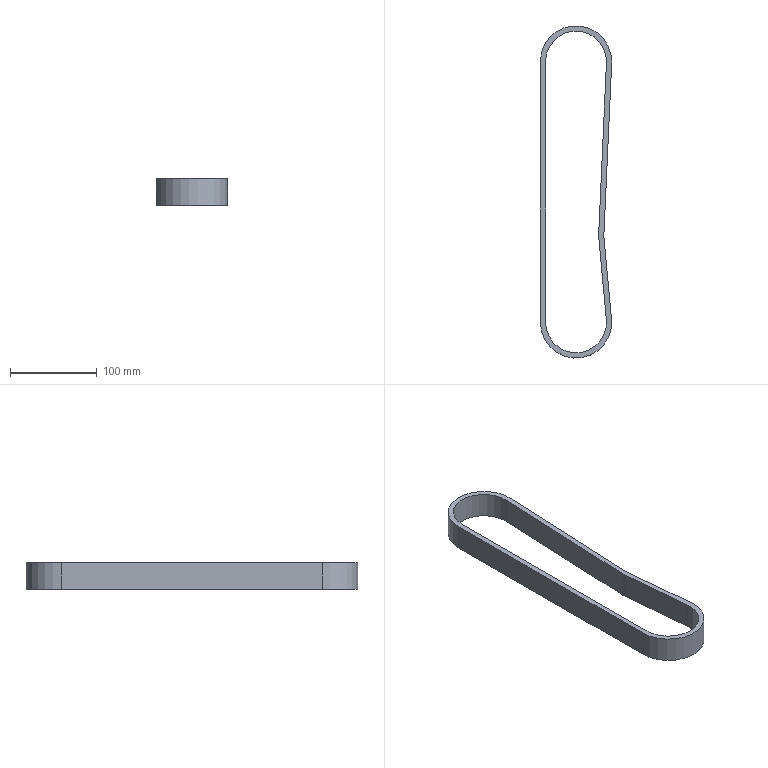Part | STEP file | belt 3-4^longitudinal seal film pull assembly 2 | 1 solid | 16 faces | box 82 x 382 x 30 mm | volume 151088 mm3 | cylinder 8 | plane 8 | commonest cylinder face diameters 40 x2 52 x2 70 x2 82 x2
STEP:
#1=CARTESIAN_POINT('',(0.,0.,0.));
#2=DIRECTION('',(0.,0.,1.));
#3=DIRECTION('',(1.,0.,0.));
#4=AXIS2_PLACEMENT_3D('',#1,#2,#3);
#5=CARTESIAN_POINT('',(32.021,100.905,-15.));
#6=VERTEX_POINT('',#5);
#7=CARTESIAN_POINT('',(32.021,100.905,15.));
#8=VERTEX_POINT('',#7);
#9=CARTESIAN_POINT('',(32.021,100.905,15.));
#10=DIRECTION('',(0.,0.,1.));
#11=VECTOR('',#10,1.);
#12=LINE('',#9,#11);
#13=CARTESIAN_POINT('',(52.,100.,15.));
#14=DIRECTION('',(0.,0.,-1.));
#15=DIRECTION('',(-1.,0.,0.));
#16=AXIS2_PLACEMENT_3D('',#13,#14,#15);
#17=CYLINDRICAL_SURFACE('',#16,20.);
#18=CARTESIAN_POINT('',(0.04528,0.));
#19=DIRECTION('',(0.,-1.));
#20=VECTOR('',#19,1.);
#21=LINE('',#18,#20);
#22=(GEOMETRIC_REPRESENTATION_CONTEXT(2)PARAMETRIC_REPRESENTATION_CONTEXT()REPRESENTATION_CONTEXT('',''));
#23=DEFINITIONAL_REPRESENTATION('',(#21),#22);
#24=PCURVE('',#17,#23);
#25=CARTESIAN_POINT('',(27.392,-1.241,15.));
#26=DIRECTION('',(-0.999,0.04527,0.));
#27=DIRECTION('',(-0.04527,-0.999,0.));
#28=AXIS2_PLACEMENT_3D('',#25,#26,#27);
#29=PLANE('',#28);
#30=CARTESIAN_POINT('',(-102.251,0.));
#31=DIRECTION('',(0.,1.));
#32=VECTOR('',#31,1.);
#33=LINE('',#30,#32);
#34=(GEOMETRIC_REPRESENTATION_CONTEXT(2)PARAMETRIC_REPRESENTATION_CONTEXT()REPRESENTATION_CONTEXT('',''));
#35=DEFINITIONAL_REPRESENTATION('',(#33),#34);
#36=PCURVE('',#29,#35);
#37=SURFACE_CURVE('',#12,(#24,#36),.PCURVE_S1.);
#38=EDGE_CURVE('',#6,#8,#37,.T.);
#39=ORIENTED_EDGE('',*,*,#38,.F.);
#40=CARTESIAN_POINT('',(32.,100.,-15.));
#41=VERTEX_POINT('',#40);
#42=CARTESIAN_POINT('',(52.,100.,-15.));
#43=DIRECTION('',(0.,0.,1.));
#44=DIRECTION('',(-1.,0.,0.));
#45=AXIS2_PLACEMENT_3D('',#42,#43,#44);
#46=CIRCLE('',#45,20.);
#47=CARTESIAN_POINT('',(6.283,30.));
#48=DIRECTION('',(-1.,0.));
#49=VECTOR('',#48,1.);
#50=LINE('',#47,#49);
#51=(GEOMETRIC_REPRESENTATION_CONTEXT(2)PARAMETRIC_REPRESENTATION_CONTEXT()REPRESENTATION_CONTEXT('',''));
#52=DEFINITIONAL_REPRESENTATION('',(#50),#51);
#53=PCURVE('',#17,#52);
#54=CARTESIAN_POINT('',(0.,0.,-15.));
#55=DIRECTION('',(0.,0.,-1.));
#56=DIRECTION('',(-1.,0.,0.));
#57=AXIS2_PLACEMENT_3D('',#54,#55,#56);
#58=PLANE('',#57);
#59=CARTESIAN_POINT('',(-32.,100.));
#60=CARTESIAN_POINT('',(-32.,65.359));
#61=CARTESIAN_POINT('',(-62.,82.679));
#62=CARTESIAN_POINT('',(-92.,100.));
#63=CARTESIAN_POINT('',(-62.,117.321));
#64=CARTESIAN_POINT('',(-32.,134.641));
#65=CARTESIAN_POINT('',(-32.,100.));
#66=(BOUNDED_CURVE()B_SPLINE_CURVE(2,(#59,#60,#61,#62,#63,#64,#65),.UNSPECIFIED.,.T.,.F.)B_SPLINE_CURVE_WITH_KNOTS((1,2,2,2,2,1),(-2.094,0.,2.094,4.189,6.283,8.378),.UNSPECIFIED.)CURVE()GEOMETRIC_REPRESENTATION_ITEM()RATIONAL_B_SPLINE_CURVE((1.,0.5,1.,0.5,1.,0.5,1.))REPRESENTATION_ITEM(''));
#67=(GEOMETRIC_REPRESENTATION_CONTEXT(2)PARAMETRIC_REPRESENTATION_CONTEXT()REPRESENTATION_CONTEXT('',''));
#68=DEFINITIONAL_REPRESENTATION('',(#66),#67);
#69=PCURVE('',#58,#68);
#70=SURFACE_CURVE('',#46,(#53,#69),.PCURVE_S1.);
#71=EDGE_CURVE('',#6,#41,#70,.T.);
#72=ORIENTED_EDGE('',*,*,#71,.T.);
#73=CARTESIAN_POINT('',(32.,100.,15.));
#74=VERTEX_POINT('',#73);
#75=CARTESIAN_POINT('',(32.,100.,15.));
#76=DIRECTION('',(0.,0.,-1.));
#77=VECTOR('',#76,1.);
#78=LINE('',#75,#77);
#79=CARTESIAN_POINT('',(0.,0.));
#80=DIRECTION('',(0.,1.));
#81=VECTOR('',#80,1.);
#82=LINE('',#79,#81);
#83=(GEOMETRIC_REPRESENTATION_CONTEXT(2)PARAMETRIC_REPRESENTATION_CONTEXT()REPRESENTATION_CONTEXT('',''));
#84=DEFINITIONAL_REPRESENTATION('',(#82),#83);
#85=PCURVE('',#17,#84);
#86=CARTESIAN_POINT('',(52.,100.,15.));
#87=DIRECTION('',(0.,0.,-1.));
#88=DIRECTION('',(-1.,0.,0.));
#89=AXIS2_PLACEMENT_3D('',#86,#87,#88);
#90=CYLINDRICAL_SURFACE('',#89,20.);
#91=CARTESIAN_POINT('',(6.283,0.));
#92=DIRECTION('',(0.,1.));
#93=VECTOR('',#92,1.);
#94=LINE('',#91,#93);
#95=(GEOMETRIC_REPRESENTATION_CONTEXT(2)PARAMETRIC_REPRESENTATION_CONTEXT()REPRESENTATION_CONTEXT('',''));
#96=DEFINITIONAL_REPRESENTATION('',(#94),#95);
#97=PCURVE('',#90,#96);
#98=SURFACE_CURVE('',#78,(#85,#97),.PCURVE_S1.);
#99=EDGE_CURVE('',#74,#41,#98,.T.);
#100=ORIENTED_EDGE('',*,*,#99,.F.);
#101=CARTESIAN_POINT('',(52.,100.,15.));
#102=DIRECTION('',(0.,0.,1.));
#103=DIRECTION('',(-1.,0.,0.));
#104=AXIS2_PLACEMENT_3D('',#101,#102,#103);
#105=CIRCLE('',#104,20.);
#106=CARTESIAN_POINT('',(6.283,0.));
#107=DIRECTION('',(-1.,0.));
#108=VECTOR('',#107,1.);
#109=LINE('',#106,#108);
#110=(GEOMETRIC_REPRESENTATION_CONTEXT(2)PARAMETRIC_REPRESENTATION_CONTEXT()REPRESENTATION_CONTEXT('',''));
#111=DEFINITIONAL_REPRESENTATION('',(#109),#110);
#112=PCURVE('',#17,#111);
#113=CARTESIAN_POINT('',(0.,0.,15.));
#114=DIRECTION('',(0.,0.,-1.));
#115=DIRECTION('',(-1.,0.,0.));
#116=AXIS2_PLACEMENT_3D('',#113,#114,#115);
#117=PLANE('',#116);
#118=CARTESIAN_POINT('',(-32.,100.));
#119=CARTESIAN_POINT('',(-32.,65.359));
#120=CARTESIAN_POINT('',(-62.,82.679));
#121=CARTESIAN_POINT('',(-92.,100.));
#122=CARTESIAN_POINT('',(-62.,117.321));
#123=CARTESIAN_POINT('',(-32.,134.641));
#124=CARTESIAN_POINT('',(-32.,100.));
#125=(BOUNDED_CURVE()B_SPLINE_CURVE(2,(#118,#119,#120,#121,#122,#123,#124),.UNSPECIFIED.,.T.,.F.)B_SPLINE_CURVE_WITH_KNOTS((1,2,2,2,2,1),(-2.094,0.,2.094,4.189,6.283,8.378),.UNSPECIFIED.)CURVE()GEOMETRIC_REPRESENTATION_ITEM()RATIONAL_B_SPLINE_CURVE((1.,0.5,1.,0.5,1.,0.5,1.))REPRESENTATION_ITEM(''));
#126=(GEOMETRIC_REPRESENTATION_CONTEXT(2)PARAMETRIC_REPRESENTATION_CONTEXT()REPRESENTATION_CONTEXT('',''));
#127=DEFINITIONAL_REPRESENTATION('',(#125),#126);
#128=PCURVE('',#117,#127);
#129=SURFACE_CURVE('',#105,(#112,#128),.PCURVE_S1.);
#130=EDGE_CURVE('',#8,#74,#129,.T.);
#131=ORIENTED_EDGE('',*,*,#130,.F.);
#132=EDGE_LOOP('',(#39,#72,#100,#131));
#133=FACE_BOUND('',#132,.F.);
#134=ADVANCED_FACE('',(#133),#17,.F.);
#135=CARTESIAN_POINT('',(26.111,97.602,15.));
#136=VERTEX_POINT('',#135);
#137=CARTESIAN_POINT('',(26.,100.,15.));
#138=VERTEX_POINT('',#137);
#139=CARTESIAN_POINT('',(52.,100.,15.));
#140=DIRECTION('',(0.,0.,-1.));
#141=DIRECTION('',(-1.,0.,0.));
#142=AXIS2_PLACEMENT_3D('',#139,#140,#141);
#143=CIRCLE('',#142,26.);
#144=CARTESIAN_POINT('',(52.,100.,15.));
#145=DIRECTION('',(0.,0.,-1.));
#146=DIRECTION('',(-1.,0.,0.));
#147=AXIS2_PLACEMENT_3D('',#144,#145,#146);
#148=CYLINDRICAL_SURFACE('',#147,26.);
#149=CARTESIAN_POINT('',(0.,0.));
#150=DIRECTION('',(1.,0.));
#151=VECTOR('',#150,1.);
#152=LINE('',#149,#151);
#153=(GEOMETRIC_REPRESENTATION_CONTEXT(2)PARAMETRIC_REPRESENTATION_CONTEXT()REPRESENTATION_CONTEXT('',''));
#154=DEFINITIONAL_REPRESENTATION('',(#152),#153);
#155=PCURVE('',#148,#154);
#156=CARTESIAN_POINT('',(-52.,100.));
#157=DIRECTION('',(1.,0.));
#158=AXIS2_PLACEMENT_2D('',#156,#157);
#159=CIRCLE('',#158,26.);
#160=(GEOMETRIC_REPRESENTATION_CONTEXT(2)PARAMETRIC_REPRESENTATION_CONTEXT()REPRESENTATION_CONTEXT('',''));
#161=DEFINITIONAL_REPRESENTATION('',(#159),#160);
#162=PCURVE('',#117,#161);
#163=SURFACE_CURVE('',#143,(#155,#162),.PCURVE_S1.);
#164=EDGE_CURVE('',#136,#138,#163,.T.);
#165=ORIENTED_EDGE('',*,*,#164,.T.);
#166=CARTESIAN_POINT('',(26.,100.,-15.));
#167=VERTEX_POINT('',#166);
#168=CARTESIAN_POINT('',(26.,100.,15.));
#169=DIRECTION('',(0.,0.,-1.));
#170=VECTOR('',#169,1.);
#171=LINE('',#168,#170);
#172=CARTESIAN_POINT('',(6.283,0.));
#173=DIRECTION('',(0.,1.));
#174=VECTOR('',#173,1.);
#175=LINE('',#172,#174);
#176=(GEOMETRIC_REPRESENTATION_CONTEXT(2)PARAMETRIC_REPRESENTATION_CONTEXT()REPRESENTATION_CONTEXT('',''));
#177=DEFINITIONAL_REPRESENTATION('',(#175),#176);
#178=PCURVE('',#148,#177);
#179=CARTESIAN_POINT('',(52.,100.,15.));
#180=DIRECTION('',(0.,0.,-1.));
#181=DIRECTION('',(-1.,0.,0.));
#182=AXIS2_PLACEMENT_3D('',#179,#180,#181);
#183=CYLINDRICAL_SURFACE('',#182,26.);
#184=CARTESIAN_POINT('',(0.,0.));
#185=DIRECTION('',(0.,1.));
#186=VECTOR('',#185,1.);
#187=LINE('',#184,#186);
#188=(GEOMETRIC_REPRESENTATION_CONTEXT(2)PARAMETRIC_REPRESENTATION_CONTEXT()REPRESENTATION_CONTEXT('',''));
#189=DEFINITIONAL_REPRESENTATION('',(#187),#188);
#190=PCURVE('',#183,#189);
#191=SURFACE_CURVE('',#171,(#178,#190),.PCURVE_S1.);
#192=EDGE_CURVE('',#138,#167,#191,.T.);
#193=ORIENTED_EDGE('',*,*,#192,.T.);
#194=CARTESIAN_POINT('',(26.111,97.602,-15.));
#195=VERTEX_POINT('',#194);
#196=CARTESIAN_POINT('',(52.,100.,-15.));
#197=DIRECTION('',(0.,0.,-1.));
#198=DIRECTION('',(-1.,0.,0.));
#199=AXIS2_PLACEMENT_3D('',#196,#197,#198);
#200=CIRCLE('',#199,26.);
#201=CARTESIAN_POINT('',(0.,30.));
#202=DIRECTION('',(1.,0.));
#203=VECTOR('',#202,1.);
#204=LINE('',#201,#203);
#205=(GEOMETRIC_REPRESENTATION_CONTEXT(2)PARAMETRIC_REPRESENTATION_CONTEXT()REPRESENTATION_CONTEXT('',''));
#206=DEFINITIONAL_REPRESENTATION('',(#204),#205);
#207=PCURVE('',#148,#206);
#208=CARTESIAN_POINT('',(-52.,100.));
#209=DIRECTION('',(1.,0.));
#210=AXIS2_PLACEMENT_2D('',#208,#209);
#211=CIRCLE('',#210,26.);
#212=(GEOMETRIC_REPRESENTATION_CONTEXT(2)PARAMETRIC_REPRESENTATION_CONTEXT()REPRESENTATION_CONTEXT('',''));
#213=DEFINITIONAL_REPRESENTATION('',(#211),#212);
#214=PCURVE('',#58,#213);
#215=SURFACE_CURVE('',#200,(#207,#214),.PCURVE_S1.);
#216=EDGE_CURVE('',#195,#167,#215,.T.);
#217=ORIENTED_EDGE('',*,*,#216,.F.);
#218=CARTESIAN_POINT('',(26.111,97.602,15.));
#219=DIRECTION('',(0.,0.,1.));
#220=VECTOR('',#219,1.);
#221=LINE('',#218,#220);
#222=CARTESIAN_POINT('',(6.191,0.));
#223=DIRECTION('',(0.,-1.));
#224=VECTOR('',#223,1.);
#225=LINE('',#222,#224);
#226=(GEOMETRIC_REPRESENTATION_CONTEXT(2)PARAMETRIC_REPRESENTATION_CONTEXT()REPRESENTATION_CONTEXT('',''));
#227=DEFINITIONAL_REPRESENTATION('',(#225),#226);
#228=PCURVE('',#148,#227);
#229=CARTESIAN_POINT('',(26.111,97.602,15.));
#230=DIRECTION('',(-0.9957,-0.09222,0.));
#231=DIRECTION('',(0.09222,-0.9957,0.));
#232=AXIS2_PLACEMENT_3D('',#229,#230,#231);
#233=PLANE('',#232);
#234=CARTESIAN_POINT('',(0.,0.));
#235=DIRECTION('',(0.,1.));
#236=VECTOR('',#235,1.);
#237=LINE('',#234,#236);
#238=(GEOMETRIC_REPRESENTATION_CONTEXT(2)PARAMETRIC_REPRESENTATION_CONTEXT()REPRESENTATION_CONTEXT('',''));
#239=DEFINITIONAL_REPRESENTATION('',(#237),#238);
#240=PCURVE('',#233,#239);
#241=SURFACE_CURVE('',#221,(#228,#240),.PCURVE_S1.);
#242=EDGE_CURVE('',#195,#136,#241,.T.);
#243=ORIENTED_EDGE('',*,*,#242,.T.);
#244=EDGE_LOOP('',(#165,#193,#217,#243));
#245=FACE_BOUND('',#244,.T.);
#246=ADVANCED_FACE('',(#245),#148,.T.);
#247=CARTESIAN_POINT('',(-41.,300.,15.));
#248=VERTEX_POINT('',#247);
#249=CARTESIAN_POINT('',(-41.,0.,15.));
#250=VERTEX_POINT('',#249);
#251=CARTESIAN_POINT('',(-41.,0.,15.));
#252=DIRECTION('',(0.,-1.,0.));
#253=VECTOR('',#252,1.);
#254=LINE('',#251,#253);
#255=CARTESIAN_POINT('',(-41.,0.,15.));
#256=DIRECTION('',(1.,0.,0.));
#257=DIRECTION('',(0.,1.,0.));
#258=AXIS2_PLACEMENT_3D('',#255,#256,#257);
#259=PLANE('',#258);
#260=CARTESIAN_POINT('',(0.,0.));
#261=DIRECTION('',(-1.,0.));
#262=VECTOR('',#261,1.);
#263=LINE('',#260,#262);
#264=(GEOMETRIC_REPRESENTATION_CONTEXT(2)PARAMETRIC_REPRESENTATION_CONTEXT()REPRESENTATION_CONTEXT('',''));
#265=DEFINITIONAL_REPRESENTATION('',(#263),#264);
#266=PCURVE('',#259,#265);
#267=CARTESIAN_POINT('',(41.,0.));
#268=DIRECTION('',(0.,-1.));
#269=VECTOR('',#268,1.);
#270=LINE('',#267,#269);
#271=(GEOMETRIC_REPRESENTATION_CONTEXT(2)PARAMETRIC_REPRESENTATION_CONTEXT()REPRESENTATION_CONTEXT('',''));
#272=DEFINITIONAL_REPRESENTATION('',(#270),#271);
#273=PCURVE('',#117,#272);
#274=SURFACE_CURVE('',#254,(#266,#273),.PCURVE_S1.);
#275=EDGE_CURVE('',#248,#250,#274,.T.);
#276=ORIENTED_EDGE('',*,*,#275,.F.);
#277=CARTESIAN_POINT('',(-41.,300.,-15.));
#278=VERTEX_POINT('',#277);
#279=CARTESIAN_POINT('',(-41.,300.,15.));
#280=DIRECTION('',(0.,0.,1.));
#281=VECTOR('',#280,1.);
#282=LINE('',#279,#281);
#283=CARTESIAN_POINT('',(300.,0.));
#284=DIRECTION('',(0.,1.));
#285=VECTOR('',#284,1.);
#286=LINE('',#283,#285);
#287=(GEOMETRIC_REPRESENTATION_CONTEXT(2)PARAMETRIC_REPRESENTATION_CONTEXT()REPRESENTATION_CONTEXT('',''));
#288=DEFINITIONAL_REPRESENTATION('',(#286),#287);
#289=PCURVE('',#259,#288);
#290=CARTESIAN_POINT('',(0.,300.,15.));
#291=DIRECTION('',(0.,0.,-1.));
#292=DIRECTION('',(-1.,0.,0.));
#293=AXIS2_PLACEMENT_3D('',#290,#291,#292);
#294=CYLINDRICAL_SURFACE('',#293,41.);
#295=CARTESIAN_POINT('',(0.,0.));
#296=DIRECTION('',(0.,-1.));
#297=VECTOR('',#296,1.);
#298=LINE('',#295,#297);
#299=(GEOMETRIC_REPRESENTATION_CONTEXT(2)PARAMETRIC_REPRESENTATION_CONTEXT()REPRESENTATION_CONTEXT('',''));
#300=DEFINITIONAL_REPRESENTATION('',(#298),#299);
#301=PCURVE('',#294,#300);
#302=SURFACE_CURVE('',#282,(#289,#301),.PCURVE_S1.);
#303=EDGE_CURVE('',#278,#248,#302,.T.);
#304=ORIENTED_EDGE('',*,*,#303,.F.);
#305=CARTESIAN_POINT('',(-41.,0.,-15.));
#306=VERTEX_POINT('',#305);
#307=CARTESIAN_POINT('',(-41.,0.,-15.));
#308=DIRECTION('',(0.,1.,0.));
#309=VECTOR('',#308,1.);
#310=LINE('',#307,#309);
#311=CARTESIAN_POINT('',(0.,-30.));
#312=DIRECTION('',(1.,0.));
#313=VECTOR('',#312,1.);
#314=LINE('',#311,#313);
#315=(GEOMETRIC_REPRESENTATION_CONTEXT(2)PARAMETRIC_REPRESENTATION_CONTEXT()REPRESENTATION_CONTEXT('',''));
#316=DEFINITIONAL_REPRESENTATION('',(#314),#315);
#317=PCURVE('',#259,#316);
#318=CARTESIAN_POINT('',(41.,0.));
#319=DIRECTION('',(0.,1.));
#320=VECTOR('',#319,1.);
#321=LINE('',#318,#320);
#322=(GEOMETRIC_REPRESENTATION_CONTEXT(2)PARAMETRIC_REPRESENTATION_CONTEXT()REPRESENTATION_CONTEXT('',''));
#323=DEFINITIONAL_REPRESENTATION('',(#321),#322);
#324=PCURVE('',#58,#323);
#325=SURFACE_CURVE('',#310,(#317,#324),.PCURVE_S1.);
#326=EDGE_CURVE('',#306,#278,#325,.T.);
#327=ORIENTED_EDGE('',*,*,#326,.F.);
#328=CARTESIAN_POINT('',(-41.,0.,15.));
#329=DIRECTION('',(0.,0.,-1.));
#330=VECTOR('',#329,1.);
#331=LINE('',#328,#330);
#332=CARTESIAN_POINT('',(0.,0.));
#333=DIRECTION('',(0.,-1.));
#334=VECTOR('',#333,1.);
#335=LINE('',#332,#334);
#336=(GEOMETRIC_REPRESENTATION_CONTEXT(2)PARAMETRIC_REPRESENTATION_CONTEXT()REPRESENTATION_CONTEXT('',''));
#337=DEFINITIONAL_REPRESENTATION('',(#335),#336);
#338=PCURVE('',#259,#337);
#339=CARTESIAN_POINT('',(0.,0.,15.));
#340=DIRECTION('',(0.,0.,-1.));
#341=DIRECTION('',(-1.,0.,0.));
#342=AXIS2_PLACEMENT_3D('',#339,#340,#341);
#343=CYLINDRICAL_SURFACE('',#342,41.);
#344=CARTESIAN_POINT('',(6.283,0.));
#345=DIRECTION('',(0.,1.));
#346=VECTOR('',#345,1.);
#347=LINE('',#344,#346);
#348=(GEOMETRIC_REPRESENTATION_CONTEXT(2)PARAMETRIC_REPRESENTATION_CONTEXT()REPRESENTATION_CONTEXT('',''));
#349=DEFINITIONAL_REPRESENTATION('',(#347),#348);
#350=PCURVE('',#343,#349);
#351=SURFACE_CURVE('',#331,(#338,#350),.PCURVE_S1.);
#352=EDGE_CURVE('',#250,#306,#351,.T.);
#353=ORIENTED_EDGE('',*,*,#352,.F.);
#354=EDGE_LOOP('',(#276,#304,#327,#353));
#355=FACE_BOUND('',#354,.T.);
#356=ADVANCED_FACE('',(#355),#259,.F.);
#357=CARTESIAN_POINT('',(40.825,3.781,-15.));
#358=VERTEX_POINT('',#357);
#359=CARTESIAN_POINT('',(0.,0.,-15.));
#360=DIRECTION('',(0.,0.,1.));
#361=DIRECTION('',(-1.,0.,0.));
#362=AXIS2_PLACEMENT_3D('',#359,#360,#361);
#363=CIRCLE('',#362,41.);
#364=CARTESIAN_POINT('',(6.283,30.));
#365=DIRECTION('',(-1.,0.));
#366=VECTOR('',#365,1.);
#367=LINE('',#364,#366);
#368=(GEOMETRIC_REPRESENTATION_CONTEXT(2)PARAMETRIC_REPRESENTATION_CONTEXT()REPRESENTATION_CONTEXT('',''));
#369=DEFINITIONAL_REPRESENTATION('',(#367),#368);
#370=PCURVE('',#343,#369);
#371=CARTESIAN_POINT('',(41.,0.));
#372=CARTESIAN_POINT('',(41.,-71.014));
#373=CARTESIAN_POINT('',(-20.5,-35.507));
#374=CARTESIAN_POINT('',(-82.,0.));
#375=CARTESIAN_POINT('',(-20.5,35.507));
#376=CARTESIAN_POINT('',(41.,71.014));
#377=CARTESIAN_POINT('',(41.,0.));
#378=(BOUNDED_CURVE()B_SPLINE_CURVE(2,(#371,#372,#373,#374,#375,#376,#377),.UNSPECIFIED.,.T.,.F.)B_SPLINE_CURVE_WITH_KNOTS((1,2,2,2,2,1),(-2.094,0.,2.094,4.189,6.283,8.378),.UNSPECIFIED.)CURVE()GEOMETRIC_REPRESENTATION_ITEM()RATIONAL_B_SPLINE_CURVE((1.,0.5,1.,0.5,1.,0.5,1.))REPRESENTATION_ITEM(''));
#379=(GEOMETRIC_REPRESENTATION_CONTEXT(2)PARAMETRIC_REPRESENTATION_CONTEXT()REPRESENTATION_CONTEXT('',''));
#380=DEFINITIONAL_REPRESENTATION('',(#378),#379);
#381=PCURVE('',#58,#380);
#382=SURFACE_CURVE('',#363,(#370,#381),.PCURVE_S1.);
#383=EDGE_CURVE('',#306,#358,#382,.T.);
#384=ORIENTED_EDGE('',*,*,#383,.T.);
#385=CARTESIAN_POINT('',(40.825,3.781,15.));
#386=VERTEX_POINT('',#385);
#387=CARTESIAN_POINT('',(40.825,3.781,15.));
#388=DIRECTION('',(0.,0.,1.));
#389=VECTOR('',#388,1.);
#390=LINE('',#387,#389);
#391=CARTESIAN_POINT('',(3.049,0.));
#392=DIRECTION('',(0.,-1.));
#393=VECTOR('',#392,1.);
#394=LINE('',#391,#393);
#395=(GEOMETRIC_REPRESENTATION_CONTEXT(2)PARAMETRIC_REPRESENTATION_CONTEXT()REPRESENTATION_CONTEXT('',''));
#396=DEFINITIONAL_REPRESENTATION('',(#394),#395);
#397=PCURVE('',#343,#396);
#398=CARTESIAN_POINT('',(40.825,3.781,15.));
#399=DIRECTION('',(-0.9957,-0.09222,0.));
#400=DIRECTION('',(0.09222,-0.9957,0.));
#401=AXIS2_PLACEMENT_3D('',#398,#399,#400);
#402=PLANE('',#401);
#403=CARTESIAN_POINT('',(0.,0.));
#404=DIRECTION('',(0.,1.));
#405=VECTOR('',#404,1.);
#406=LINE('',#403,#405);
#407=(GEOMETRIC_REPRESENTATION_CONTEXT(2)PARAMETRIC_REPRESENTATION_CONTEXT()REPRESENTATION_CONTEXT('',''));
#408=DEFINITIONAL_REPRESENTATION('',(#406),#407);
#409=PCURVE('',#402,#408);
#410=SURFACE_CURVE('',#390,(#397,#409),.PCURVE_S1.);
#411=EDGE_CURVE('',#358,#386,#410,.T.);
#412=ORIENTED_EDGE('',*,*,#411,.T.);
#413=CARTESIAN_POINT('',(0.,0.,15.));
#414=DIRECTION('',(0.,0.,-1.));
#415=DIRECTION('',(-1.,0.,0.));
#416=AXIS2_PLACEMENT_3D('',#413,#414,#415);
#417=CIRCLE('',#416,41.);
#418=CARTESIAN_POINT('',(0.,0.));
#419=DIRECTION('',(1.,0.));
#420=VECTOR('',#419,1.);
#421=LINE('',#418,#420);
#422=(GEOMETRIC_REPRESENTATION_CONTEXT(2)PARAMETRIC_REPRESENTATION_CONTEXT()REPRESENTATION_CONTEXT('',''));
#423=DEFINITIONAL_REPRESENTATION('',(#421),#422);
#424=PCURVE('',#343,#423);
#425=CARTESIAN_POINT('',(0.,0.));
#426=DIRECTION('',(1.,0.));
#427=AXIS2_PLACEMENT_2D('',#425,#426);
#428=CIRCLE('',#427,41.);
#429=(GEOMETRIC_REPRESENTATION_CONTEXT(2)PARAMETRIC_REPRESENTATION_CONTEXT()REPRESENTATION_CONTEXT('',''));
#430=DEFINITIONAL_REPRESENTATION('',(#428),#429);
#431=PCURVE('',#117,#430);
#432=SURFACE_CURVE('',#417,(#424,#431),.PCURVE_S1.);
#433=EDGE_CURVE('',#386,#250,#432,.T.);
#434=ORIENTED_EDGE('',*,*,#433,.T.);
#435=ORIENTED_EDGE('',*,*,#352,.T.);
#436=EDGE_LOOP('',(#384,#412,#434,#435));
#437=FACE_BOUND('',#436,.T.);
#438=ADVANCED_FACE('',(#437),#343,.T.);
#439=ORIENTED_EDGE('',*,*,#130,.F.);
#440=CARTESIAN_POINT('',(40.958,298.144,15.));
#441=VERTEX_POINT('',#440);
#442=CARTESIAN_POINT('',(40.958,298.144,15.));
#443=DIRECTION('',(-0.04527,-0.999,0.));
#444=VECTOR('',#443,1.);
#445=LINE('',#442,#444);
#446=CARTESIAN_POINT('',(-40.958,298.144));
#447=DIRECTION('',(0.04527,-0.999));
#448=VECTOR('',#447,1.);
#449=LINE('',#446,#448);
#450=(GEOMETRIC_REPRESENTATION_CONTEXT(2)PARAMETRIC_REPRESENTATION_CONTEXT()REPRESENTATION_CONTEXT('',''));
#451=DEFINITIONAL_REPRESENTATION('',(#449),#450);
#452=PCURVE('',#117,#451);
#453=CARTESIAN_POINT('',(-299.692,0.));
#454=DIRECTION('',(1.,0.));
#455=VECTOR('',#454,1.);
#456=LINE('',#453,#455);
#457=(GEOMETRIC_REPRESENTATION_CONTEXT(2)PARAMETRIC_REPRESENTATION_CONTEXT()REPRESENTATION_CONTEXT('',''));
#458=DEFINITIONAL_REPRESENTATION('',(#456),#457);
#459=PCURVE('',#29,#458);
#460=SURFACE_CURVE('',#445,(#452,#459),.PCURVE_S1.);
#461=EDGE_CURVE('',#441,#8,#460,.T.);
#462=ORIENTED_EDGE('',*,*,#461,.F.);
#463=CARTESIAN_POINT('',(0.,300.,15.));
#464=DIRECTION('',(0.,0.,-1.));
#465=DIRECTION('',(-1.,0.,0.));
#466=AXIS2_PLACEMENT_3D('',#463,#464,#465);
#467=CIRCLE('',#466,41.);
#468=CARTESIAN_POINT('',(0.,300.));
#469=DIRECTION('',(1.,0.));
#470=AXIS2_PLACEMENT_2D('',#468,#469);
#471=CIRCLE('',#470,41.);
#472=(GEOMETRIC_REPRESENTATION_CONTEXT(2)PARAMETRIC_REPRESENTATION_CONTEXT()REPRESENTATION_CONTEXT('',''));
#473=DEFINITIONAL_REPRESENTATION('',(#471),#472);
#474=PCURVE('',#117,#473);
#475=CARTESIAN_POINT('',(0.,0.));
#476=DIRECTION('',(1.,0.));
#477=VECTOR('',#476,1.);
#478=LINE('',#475,#477);
#479=(GEOMETRIC_REPRESENTATION_CONTEXT(2)PARAMETRIC_REPRESENTATION_CONTEXT()REPRESENTATION_CONTEXT('',''));
#480=DEFINITIONAL_REPRESENTATION('',(#478),#479);
#481=PCURVE('',#294,#480);
#482=SURFACE_CURVE('',#467,(#474,#481),.PCURVE_S1.);
#483=EDGE_CURVE('',#248,#441,#482,.T.);
#484=ORIENTED_EDGE('',*,*,#483,.F.);
#485=ORIENTED_EDGE('',*,*,#275,.T.);
#486=ORIENTED_EDGE('',*,*,#433,.F.);
#487=CARTESIAN_POINT('',(32.085,98.156,15.));
#488=VERTEX_POINT('',#487);
#489=CARTESIAN_POINT('',(32.085,98.156,15.));
#490=DIRECTION('',(0.09222,-0.9957,0.));
#491=VECTOR('',#490,1.);
#492=LINE('',#489,#491);
#493=CARTESIAN_POINT('',(-32.085,98.156));
#494=DIRECTION('',(-0.09222,-0.9957));
#495=VECTOR('',#494,1.);
#496=LINE('',#493,#495);
#497=(GEOMETRIC_REPRESENTATION_CONTEXT(2)PARAMETRIC_REPRESENTATION_CONTEXT()REPRESENTATION_CONTEXT('',''));
#498=DEFINITIONAL_REPRESENTATION('',(#496),#497);
#499=PCURVE('',#117,#498);
#500=CARTESIAN_POINT('',(-94.779,0.));
#501=DIRECTION('',(1.,0.));
#502=VECTOR('',#501,1.);
#503=LINE('',#500,#502);
#504=(GEOMETRIC_REPRESENTATION_CONTEXT(2)PARAMETRIC_REPRESENTATION_CONTEXT()REPRESENTATION_CONTEXT('',''));
#505=DEFINITIONAL_REPRESENTATION('',(#503),#504);
#506=PCURVE('',#402,#505);
#507=SURFACE_CURVE('',#492,(#499,#506),.PCURVE_S1.);
#508=EDGE_CURVE('',#488,#386,#507,.T.);
#509=ORIENTED_EDGE('',*,*,#508,.F.);
#510=CARTESIAN_POINT('',(52.,100.,15.));
#511=DIRECTION('',(0.,0.,1.));
#512=DIRECTION('',(-1.,0.,0.));
#513=AXIS2_PLACEMENT_3D('',#510,#511,#512);
#514=CIRCLE('',#513,20.);
#515=CARTESIAN_POINT('',(-32.,100.));
#516=CARTESIAN_POINT('',(-32.,65.359));
#517=CARTESIAN_POINT('',(-62.,82.679));
#518=CARTESIAN_POINT('',(-92.,100.));
#519=CARTESIAN_POINT('',(-62.,117.321));
#520=CARTESIAN_POINT('',(-32.,134.641));
#521=CARTESIAN_POINT('',(-32.,100.));
#522=(BOUNDED_CURVE()B_SPLINE_CURVE(2,(#515,#516,#517,#518,#519,#520,#521),.UNSPECIFIED.,.T.,.F.)B_SPLINE_CURVE_WITH_KNOTS((1,2,2,2,2,1),(-2.094,0.,2.094,4.189,6.283,8.378),.UNSPECIFIED.)CURVE()GEOMETRIC_REPRESENTATION_ITEM()RATIONAL_B_SPLINE_CURVE((1.,0.5,1.,0.5,1.,0.5,1.))REPRESENTATION_ITEM(''));
#523=(GEOMETRIC_REPRESENTATION_CONTEXT(2)PARAMETRIC_REPRESENTATION_CONTEXT()REPRESENTATION_CONTEXT('',''));
#524=DEFINITIONAL_REPRESENTATION('',(#522),#523);
#525=PCURVE('',#117,#524);
#526=CARTESIAN_POINT('',(6.283,0.));
#527=DIRECTION('',(-1.,0.));
#528=VECTOR('',#527,1.);
#529=LINE('',#526,#528);
#530=(GEOMETRIC_REPRESENTATION_CONTEXT(2)PARAMETRIC_REPRESENTATION_CONTEXT()REPRESENTATION_CONTEXT('',''));
#531=DEFINITIONAL_REPRESENTATION('',(#529),#530);
#532=PCURVE('',#90,#531);
#533=SURFACE_CURVE('',#514,(#525,#532),.PCURVE_S1.);
#534=EDGE_CURVE('',#74,#488,#533,.T.);
#535=ORIENTED_EDGE('',*,*,#534,.F.);
#536=EDGE_LOOP('',(#439,#462,#484,#485,#486,#509,#535));
#537=FACE_BOUND('',#536,.T.);
#538=CARTESIAN_POINT('',(34.964,298.416,15.));
#539=VERTEX_POINT('',#538);
#540=CARTESIAN_POINT('',(-35.,300.,15.));
#541=VERTEX_POINT('',#540);
#542=CARTESIAN_POINT('',(0.,300.,15.));
#543=DIRECTION('',(0.,0.,1.));
#544=DIRECTION('',(-1.,0.,0.));
#545=AXIS2_PLACEMENT_3D('',#542,#543,#544);
#546=CIRCLE('',#545,35.);
#547=CARTESIAN_POINT('',(35.,300.));
#548=CARTESIAN_POINT('',(35.,239.378));
#549=CARTESIAN_POINT('',(-17.5,269.689));
#550=CARTESIAN_POINT('',(-70.,300.));
#551=CARTESIAN_POINT('',(-17.5,330.311));
#552=CARTESIAN_POINT('',(35.,360.622));
#553=CARTESIAN_POINT('',(35.,300.));
#554=(BOUNDED_CURVE()B_SPLINE_CURVE(2,(#547,#548,#549,#550,#551,#552,#553),.UNSPECIFIED.,.T.,.F.)B_SPLINE_CURVE_WITH_KNOTS((1,2,2,2,2,1),(-2.094,0.,2.094,4.189,6.283,8.378),.UNSPECIFIED.)CURVE()GEOMETRIC_REPRESENTATION_ITEM()RATIONAL_B_SPLINE_CURVE((1.,0.5,1.,0.5,1.,0.5,1.))REPRESENTATION_ITEM(''));
#555=(GEOMETRIC_REPRESENTATION_CONTEXT(2)PARAMETRIC_REPRESENTATION_CONTEXT()REPRESENTATION_CONTEXT('',''));
#556=DEFINITIONAL_REPRESENTATION('',(#554),#555);
#557=PCURVE('',#117,#556);
#558=CARTESIAN_POINT('',(0.,300.,15.));
#559=DIRECTION('',(0.,0.,-1.));
#560=DIRECTION('',(-1.,0.,0.));
#561=AXIS2_PLACEMENT_3D('',#558,#559,#560);
#562=CYLINDRICAL_SURFACE('',#561,35.);
#563=CARTESIAN_POINT('',(6.283,0.));
#564=DIRECTION('',(-1.,0.));
#565=VECTOR('',#564,1.);
#566=LINE('',#563,#565);
#567=(GEOMETRIC_REPRESENTATION_CONTEXT(2)PARAMETRIC_REPRESENTATION_CONTEXT()REPRESENTATION_CONTEXT('',''));
#568=DEFINITIONAL_REPRESENTATION('',(#566),#567);
#569=PCURVE('',#562,#568);
#570=SURFACE_CURVE('',#546,(#557,#569),.PCURVE_S1.);
#571=EDGE_CURVE('',#539,#541,#570,.T.);
#572=ORIENTED_EDGE('',*,*,#571,.F.);
#573=CARTESIAN_POINT('',(26.027,101.177,15.));
#574=VERTEX_POINT('',#573);
#575=CARTESIAN_POINT('',(26.027,101.177,15.));
#576=DIRECTION('',(0.04527,0.999,0.));
#577=VECTOR('',#576,1.);
#578=LINE('',#575,#577);
#579=CARTESIAN_POINT('',(-26.027,101.177));
#580=DIRECTION('',(-0.04527,0.999));
#581=VECTOR('',#580,1.);
#582=LINE('',#579,#581);
#583=(GEOMETRIC_REPRESENTATION_CONTEXT(2)PARAMETRIC_REPRESENTATION_CONTEXT()REPRESENTATION_CONTEXT('',''));
#584=DEFINITIONAL_REPRESENTATION('',(#582),#583);
#585=PCURVE('',#117,#584);
#586=CARTESIAN_POINT('',(34.964,298.416,15.));
#587=DIRECTION('',(-0.999,0.04527,0.));
#588=DIRECTION('',(-0.04527,-0.999,0.));
#589=AXIS2_PLACEMENT_3D('',#586,#587,#588);
#590=PLANE('',#589);
#591=CARTESIAN_POINT('',(197.441,0.));
#592=DIRECTION('',(-1.,0.));
#593=VECTOR('',#592,1.);
#594=LINE('',#591,#593);
#595=(GEOMETRIC_REPRESENTATION_CONTEXT(2)PARAMETRIC_REPRESENTATION_CONTEXT()REPRESENTATION_CONTEXT('',''));
#596=DEFINITIONAL_REPRESENTATION('',(#594),#595);
#597=PCURVE('',#590,#596);
#598=SURFACE_CURVE('',#578,(#585,#597),.PCURVE_S1.);
#599=EDGE_CURVE('',#574,#539,#598,.T.);
#600=ORIENTED_EDGE('',*,*,#599,.F.);
#601=CARTESIAN_POINT('',(52.,100.,15.));
#602=DIRECTION('',(0.,0.,-1.));
#603=DIRECTION('',(-1.,0.,0.));
#604=AXIS2_PLACEMENT_3D('',#601,#602,#603);
#605=CIRCLE('',#604,26.);
#606=CARTESIAN_POINT('',(-52.,100.));
#607=DIRECTION('',(1.,0.));
#608=AXIS2_PLACEMENT_2D('',#606,#607);
#609=CIRCLE('',#608,26.);
#610=(GEOMETRIC_REPRESENTATION_CONTEXT(2)PARAMETRIC_REPRESENTATION_CONTEXT()REPRESENTATION_CONTEXT('',''));
#611=DEFINITIONAL_REPRESENTATION('',(#609),#610);
#612=PCURVE('',#117,#611);
#613=CARTESIAN_POINT('',(0.,0.));
#614=DIRECTION('',(1.,0.));
#615=VECTOR('',#614,1.);
#616=LINE('',#613,#615);
#617=(GEOMETRIC_REPRESENTATION_CONTEXT(2)PARAMETRIC_REPRESENTATION_CONTEXT()REPRESENTATION_CONTEXT('',''));
#618=DEFINITIONAL_REPRESENTATION('',(#616),#617);
#619=PCURVE('',#183,#618);
#620=SURFACE_CURVE('',#605,(#612,#619),.PCURVE_S1.);
#621=EDGE_CURVE('',#138,#574,#620,.T.);
#622=ORIENTED_EDGE('',*,*,#621,.F.);
#623=ORIENTED_EDGE('',*,*,#164,.F.);
#624=CARTESIAN_POINT('',(34.851,3.228,15.));
#625=VERTEX_POINT('',#624);
#626=CARTESIAN_POINT('',(34.851,3.228,15.));
#627=DIRECTION('',(-0.09222,0.9957,0.));
#628=VECTOR('',#627,1.);
#629=LINE('',#626,#628);
#630=CARTESIAN_POINT('',(-34.851,3.228));
#631=DIRECTION('',(0.09222,0.9957));
#632=VECTOR('',#631,1.);
#633=LINE('',#630,#632);
#634=(GEOMETRIC_REPRESENTATION_CONTEXT(2)PARAMETRIC_REPRESENTATION_CONTEXT()REPRESENTATION_CONTEXT('',''));
#635=DEFINITIONAL_REPRESENTATION('',(#633),#634);
#636=PCURVE('',#117,#635);
#637=CARTESIAN_POINT('',(94.779,0.));
#638=DIRECTION('',(-1.,0.));
#639=VECTOR('',#638,1.);
#640=LINE('',#637,#639);
#641=(GEOMETRIC_REPRESENTATION_CONTEXT(2)PARAMETRIC_REPRESENTATION_CONTEXT()REPRESENTATION_CONTEXT('',''));
#642=DEFINITIONAL_REPRESENTATION('',(#640),#641);
#643=PCURVE('',#233,#642);
#644=SURFACE_CURVE('',#629,(#636,#643),.PCURVE_S1.);
#645=EDGE_CURVE('',#625,#136,#644,.T.);
#646=ORIENTED_EDGE('',*,*,#645,.F.);
#647=CARTESIAN_POINT('',(-35.,0.,15.));
#648=VERTEX_POINT('',#647);
#649=CARTESIAN_POINT('',(0.,0.,15.));
#650=DIRECTION('',(0.,0.,1.));
#651=DIRECTION('',(-1.,0.,0.));
#652=AXIS2_PLACEMENT_3D('',#649,#650,#651);
#653=CIRCLE('',#652,35.);
#654=CARTESIAN_POINT('',(35.,0.));
#655=CARTESIAN_POINT('',(35.,-60.622));
#656=CARTESIAN_POINT('',(-17.5,-30.311));
#657=CARTESIAN_POINT('',(-70.,0.));
#658=CARTESIAN_POINT('',(-17.5,30.311));
#659=CARTESIAN_POINT('',(35.,60.622));
#660=CARTESIAN_POINT('',(35.,0.));
#661=(BOUNDED_CURVE()B_SPLINE_CURVE(2,(#654,#655,#656,#657,#658,#659,#660),.UNSPECIFIED.,.T.,.F.)B_SPLINE_CURVE_WITH_KNOTS((1,2,2,2,2,1),(-2.094,0.,2.094,4.189,6.283,8.378),.UNSPECIFIED.)CURVE()GEOMETRIC_REPRESENTATION_ITEM()RATIONAL_B_SPLINE_CURVE((1.,0.5,1.,0.5,1.,0.5,1.))REPRESENTATION_ITEM(''));
#662=(GEOMETRIC_REPRESENTATION_CONTEXT(2)PARAMETRIC_REPRESENTATION_CONTEXT()REPRESENTATION_CONTEXT('',''));
#663=DEFINITIONAL_REPRESENTATION('',(#661),#662);
#664=PCURVE('',#117,#663);
#665=CARTESIAN_POINT('',(0.,0.,15.));
#666=DIRECTION('',(0.,0.,-1.));
#667=DIRECTION('',(-1.,0.,0.));
#668=AXIS2_PLACEMENT_3D('',#665,#666,#667);
#669=CYLINDRICAL_SURFACE('',#668,35.);
#670=CARTESIAN_POINT('',(6.283,0.));
#671=DIRECTION('',(-1.,0.));
#672=VECTOR('',#671,1.);
#673=LINE('',#670,#672);
#674=(GEOMETRIC_REPRESENTATION_CONTEXT(2)PARAMETRIC_REPRESENTATION_CONTEXT()REPRESENTATION_CONTEXT('',''));
#675=DEFINITIONAL_REPRESENTATION('',(#673),#674);
#676=PCURVE('',#669,#675);
#677=SURFACE_CURVE('',#653,(#664,#676),.PCURVE_S1.);
#678=EDGE_CURVE('',#648,#625,#677,.T.);
#679=ORIENTED_EDGE('',*,*,#678,.F.);
#680=CARTESIAN_POINT('',(-35.,0.,15.));
#681=DIRECTION('',(0.,-1.,0.));
#682=VECTOR('',#681,1.);
#683=LINE('',#680,#682);
#684=CARTESIAN_POINT('',(35.,0.));
#685=DIRECTION('',(0.,-1.));
#686=VECTOR('',#685,1.);
#687=LINE('',#684,#686);
#688=(GEOMETRIC_REPRESENTATION_CONTEXT(2)PARAMETRIC_REPRESENTATION_CONTEXT()REPRESENTATION_CONTEXT('',''));
#689=DEFINITIONAL_REPRESENTATION('',(#687),#688);
#690=PCURVE('',#117,#689);
#691=CARTESIAN_POINT('',(-35.,0.,15.));
#692=DIRECTION('',(1.,0.,0.));
#693=DIRECTION('',(0.,1.,0.));
#694=AXIS2_PLACEMENT_3D('',#691,#692,#693);
#695=PLANE('',#694);
#696=CARTESIAN_POINT('',(0.,0.));
#697=DIRECTION('',(-1.,0.));
#698=VECTOR('',#697,1.);
#699=LINE('',#696,#698);
#700=(GEOMETRIC_REPRESENTATION_CONTEXT(2)PARAMETRIC_REPRESENTATION_CONTEXT()REPRESENTATION_CONTEXT('',''));
#701=DEFINITIONAL_REPRESENTATION('',(#699),#700);
#702=PCURVE('',#695,#701);
#703=SURFACE_CURVE('',#683,(#690,#702),.PCURVE_S1.);
#704=EDGE_CURVE('',#541,#648,#703,.T.);
#705=ORIENTED_EDGE('',*,*,#704,.F.);
#706=EDGE_LOOP('',(#572,#600,#622,#623,#646,#679,#705));
#707=FACE_BOUND('',#706,.T.);
#708=ADVANCED_FACE('',(#537,#707),#117,.F.);
#709=CARTESIAN_POINT('',(40.958,298.144,-15.));
#710=VERTEX_POINT('',#709);
#711=CARTESIAN_POINT('',(0.,300.,-15.));
#712=DIRECTION('',(0.,0.,1.));
#713=DIRECTION('',(-1.,0.,0.));
#714=AXIS2_PLACEMENT_3D('',#711,#712,#713);
#715=CIRCLE('',#714,41.);
#716=CARTESIAN_POINT('',(6.283,30.));
#717=DIRECTION('',(-1.,0.));
#718=VECTOR('',#717,1.);
#719=LINE('',#716,#718);
#720=(GEOMETRIC_REPRESENTATION_CONTEXT(2)PARAMETRIC_REPRESENTATION_CONTEXT()REPRESENTATION_CONTEXT('',''));
#721=DEFINITIONAL_REPRESENTATION('',(#719),#720);
#722=PCURVE('',#294,#721);
#723=CARTESIAN_POINT('',(41.,300.));
#724=CARTESIAN_POINT('',(41.,228.986));
#725=CARTESIAN_POINT('',(-20.5,264.493));
#726=CARTESIAN_POINT('',(-82.,300.));
#727=CARTESIAN_POINT('',(-20.5,335.507));
#728=CARTESIAN_POINT('',(41.,371.014));
#729=CARTESIAN_POINT('',(41.,300.));
#730=(BOUNDED_CURVE()B_SPLINE_CURVE(2,(#723,#724,#725,#726,#727,#728,#729),.UNSPECIFIED.,.T.,.F.)B_SPLINE_CURVE_WITH_KNOTS((1,2,2,2,2,1),(-2.094,0.,2.094,4.189,6.283,8.378),.UNSPECIFIED.)CURVE()GEOMETRIC_REPRESENTATION_ITEM()RATIONAL_B_SPLINE_CURVE((1.,0.5,1.,0.5,1.,0.5,1.))REPRESENTATION_ITEM(''));
#731=(GEOMETRIC_REPRESENTATION_CONTEXT(2)PARAMETRIC_REPRESENTATION_CONTEXT()REPRESENTATION_CONTEXT('',''));
#732=DEFINITIONAL_REPRESENTATION('',(#730),#731);
#733=PCURVE('',#58,#732);
#734=SURFACE_CURVE('',#715,(#722,#733),.PCURVE_S1.);
#735=EDGE_CURVE('',#710,#278,#734,.T.);
#736=ORIENTED_EDGE('',*,*,#735,.T.);
#737=ORIENTED_EDGE('',*,*,#303,.T.);
#738=ORIENTED_EDGE('',*,*,#483,.T.);
#739=CARTESIAN_POINT('',(40.958,298.144,15.));
#740=DIRECTION('',(0.,0.,-1.));
#741=VECTOR('',#740,1.);
#742=LINE('',#739,#741);
#743=CARTESIAN_POINT('',(3.187,0.));
#744=DIRECTION('',(0.,1.));
#745=VECTOR('',#744,1.);
#746=LINE('',#743,#745);
#747=(GEOMETRIC_REPRESENTATION_CONTEXT(2)PARAMETRIC_REPRESENTATION_CONTEXT()REPRESENTATION_CONTEXT('',''));
#748=DEFINITIONAL_REPRESENTATION('',(#746),#747);
#749=PCURVE('',#294,#748);
#750=CARTESIAN_POINT('',(-299.692,0.));
#751=DIRECTION('',(0.,-1.));
#752=VECTOR('',#751,1.);
#753=LINE('',#750,#752);
#754=(GEOMETRIC_REPRESENTATION_CONTEXT(2)PARAMETRIC_REPRESENTATION_CONTEXT()REPRESENTATION_CONTEXT('',''));
#755=DEFINITIONAL_REPRESENTATION('',(#753),#754);
#756=PCURVE('',#29,#755);
#757=SURFACE_CURVE('',#742,(#749,#756),.PCURVE_S1.);
#758=EDGE_CURVE('',#441,#710,#757,.T.);
#759=ORIENTED_EDGE('',*,*,#758,.T.);
#760=EDGE_LOOP('',(#736,#737,#738,#759));
#761=FACE_BOUND('',#760,.T.);
#762=ADVANCED_FACE('',(#761),#294,.T.);
#763=ORIENTED_EDGE('',*,*,#735,.F.);
#764=CARTESIAN_POINT('',(40.958,298.144,-15.));
#765=DIRECTION('',(-0.04527,-0.999,0.));
#766=VECTOR('',#765,1.);
#767=LINE('',#764,#766);
#768=CARTESIAN_POINT('',(-40.958,298.144));
#769=DIRECTION('',(0.04527,-0.999));
#770=VECTOR('',#769,1.);
#771=LINE('',#768,#770);
#772=(GEOMETRIC_REPRESENTATION_CONTEXT(2)PARAMETRIC_REPRESENTATION_CONTEXT()REPRESENTATION_CONTEXT('',''));
#773=DEFINITIONAL_REPRESENTATION('',(#771),#772);
#774=PCURVE('',#58,#773);
#775=CARTESIAN_POINT('',(-299.692,-30.));
#776=DIRECTION('',(1.,0.));
#777=VECTOR('',#776,1.);
#778=LINE('',#775,#777);
#779=(GEOMETRIC_REPRESENTATION_CONTEXT(2)PARAMETRIC_REPRESENTATION_CONTEXT()REPRESENTATION_CONTEXT('',''));
#780=DEFINITIONAL_REPRESENTATION('',(#778),#779);
#781=PCURVE('',#29,#780);
#782=SURFACE_CURVE('',#767,(#774,#781),.PCURVE_S1.);
#783=EDGE_CURVE('',#710,#6,#782,.T.);
#784=ORIENTED_EDGE('',*,*,#783,.T.);
#785=ORIENTED_EDGE('',*,*,#71,.T.);
#786=CARTESIAN_POINT('',(32.085,98.156,-15.));
#787=VERTEX_POINT('',#786);
#788=CARTESIAN_POINT('',(52.,100.,-15.));
#789=DIRECTION('',(0.,0.,1.));
#790=DIRECTION('',(-1.,0.,0.));
#791=AXIS2_PLACEMENT_3D('',#788,#789,#790);
#792=CIRCLE('',#791,20.);
#793=CARTESIAN_POINT('',(-32.,100.));
#794=CARTESIAN_POINT('',(-32.,65.359));
#795=CARTESIAN_POINT('',(-62.,82.679));
#796=CARTESIAN_POINT('',(-92.,100.));
#797=CARTESIAN_POINT('',(-62.,117.321));
#798=CARTESIAN_POINT('',(-32.,134.641));
#799=CARTESIAN_POINT('',(-32.,100.));
#800=(BOUNDED_CURVE()B_SPLINE_CURVE(2,(#793,#794,#795,#796,#797,#798,#799),.UNSPECIFIED.,.T.,.F.)B_SPLINE_CURVE_WITH_KNOTS((1,2,2,2,2,1),(-2.094,0.,2.094,4.189,6.283,8.378),.UNSPECIFIED.)CURVE()GEOMETRIC_REPRESENTATION_ITEM()RATIONAL_B_SPLINE_CURVE((1.,0.5,1.,0.5,1.,0.5,1.))REPRESENTATION_ITEM(''));
#801=(GEOMETRIC_REPRESENTATION_CONTEXT(2)PARAMETRIC_REPRESENTATION_CONTEXT()REPRESENTATION_CONTEXT('',''));
#802=DEFINITIONAL_REPRESENTATION('',(#800),#801);
#803=PCURVE('',#58,#802);
#804=CARTESIAN_POINT('',(6.283,30.));
#805=DIRECTION('',(-1.,0.));
#806=VECTOR('',#805,1.);
#807=LINE('',#804,#806);
#808=(GEOMETRIC_REPRESENTATION_CONTEXT(2)PARAMETRIC_REPRESENTATION_CONTEXT()REPRESENTATION_CONTEXT('',''));
#809=DEFINITIONAL_REPRESENTATION('',(#807),#808);
#810=PCURVE('',#90,#809);
#811=SURFACE_CURVE('',#792,(#803,#810),.PCURVE_S1.);
#812=EDGE_CURVE('',#41,#787,#811,.T.);
#813=ORIENTED_EDGE('',*,*,#812,.T.);
#814=CARTESIAN_POINT('',(32.085,98.156,-15.));
#815=DIRECTION('',(0.09222,-0.9957,0.));
#816=VECTOR('',#815,1.);
#817=LINE('',#814,#816);
#818=CARTESIAN_POINT('',(-32.085,98.156));
#819=DIRECTION('',(-0.09222,-0.9957));
#820=VECTOR('',#819,1.);
#821=LINE('',#818,#820);
#822=(GEOMETRIC_REPRESENTATION_CONTEXT(2)PARAMETRIC_REPRESENTATION_CONTEXT()REPRESENTATION_CONTEXT('',''));
#823=DEFINITIONAL_REPRESENTATION('',(#821),#822);
#824=PCURVE('',#58,#823);
#825=CARTESIAN_POINT('',(-94.779,-30.));
#826=DIRECTION('',(1.,0.));
#827=VECTOR('',#826,1.);
#828=LINE('',#825,#827);
#829=(GEOMETRIC_REPRESENTATION_CONTEXT(2)PARAMETRIC_REPRESENTATION_CONTEXT()REPRESENTATION_CONTEXT('',''));
#830=DEFINITIONAL_REPRESENTATION('',(#828),#829);
#831=PCURVE('',#402,#830);
#832=SURFACE_CURVE('',#817,(#824,#831),.PCURVE_S1.);
#833=EDGE_CURVE('',#787,#358,#832,.T.);
#834=ORIENTED_EDGE('',*,*,#833,.T.);
#835=ORIENTED_EDGE('',*,*,#383,.F.);
#836=ORIENTED_EDGE('',*,*,#326,.T.);
#837=EDGE_LOOP('',(#763,#784,#785,#813,#834,#835,#836));
#838=FACE_BOUND('',#837,.T.);
#839=ORIENTED_EDGE('',*,*,#216,.T.);
#840=CARTESIAN_POINT('',(26.027,101.177,-15.));
#841=VERTEX_POINT('',#840);
#842=CARTESIAN_POINT('',(52.,100.,-15.));
#843=DIRECTION('',(0.,0.,-1.));
#844=DIRECTION('',(-1.,0.,0.));
#845=AXIS2_PLACEMENT_3D('',#842,#843,#844);
#846=CIRCLE('',#845,26.);
#847=CARTESIAN_POINT('',(-52.,100.));
#848=DIRECTION('',(1.,0.));
#849=AXIS2_PLACEMENT_2D('',#847,#848);
#850=CIRCLE('',#849,26.);
#851=(GEOMETRIC_REPRESENTATION_CONTEXT(2)PARAMETRIC_REPRESENTATION_CONTEXT()REPRESENTATION_CONTEXT('',''));
#852=DEFINITIONAL_REPRESENTATION('',(#850),#851);
#853=PCURVE('',#58,#852);
#854=CARTESIAN_POINT('',(0.,30.));
#855=DIRECTION('',(1.,0.));
#856=VECTOR('',#855,1.);
#857=LINE('',#854,#856);
#858=(GEOMETRIC_REPRESENTATION_CONTEXT(2)PARAMETRIC_REPRESENTATION_CONTEXT()REPRESENTATION_CONTEXT('',''));
#859=DEFINITIONAL_REPRESENTATION('',(#857),#858);
#860=PCURVE('',#183,#859);
#861=SURFACE_CURVE('',#846,(#853,#860),.PCURVE_S1.);
#862=EDGE_CURVE('',#167,#841,#861,.T.);
#863=ORIENTED_EDGE('',*,*,#862,.T.);
#864=CARTESIAN_POINT('',(34.964,298.416,-15.));
#865=VERTEX_POINT('',#864);
#866=CARTESIAN_POINT('',(26.027,101.177,-15.));
#867=DIRECTION('',(0.04527,0.999,0.));
#868=VECTOR('',#867,1.);
#869=LINE('',#866,#868);
#870=CARTESIAN_POINT('',(-26.027,101.177));
#871=DIRECTION('',(-0.04527,0.999));
#872=VECTOR('',#871,1.);
#873=LINE('',#870,#872);
#874=(GEOMETRIC_REPRESENTATION_CONTEXT(2)PARAMETRIC_REPRESENTATION_CONTEXT()REPRESENTATION_CONTEXT('',''));
#875=DEFINITIONAL_REPRESENTATION('',(#873),#874);
#876=PCURVE('',#58,#875);
#877=CARTESIAN_POINT('',(197.441,-30.));
#878=DIRECTION('',(-1.,0.));
#879=VECTOR('',#878,1.);
#880=LINE('',#877,#879);
#881=(GEOMETRIC_REPRESENTATION_CONTEXT(2)PARAMETRIC_REPRESENTATION_CONTEXT()REPRESENTATION_CONTEXT('',''));
#882=DEFINITIONAL_REPRESENTATION('',(#880),#881);
#883=PCURVE('',#590,#882);
#884=SURFACE_CURVE('',#869,(#876,#883),.PCURVE_S1.);
#885=EDGE_CURVE('',#841,#865,#884,.T.);
#886=ORIENTED_EDGE('',*,*,#885,.T.);
#887=CARTESIAN_POINT('',(-35.,300.,-15.));
#888=VERTEX_POINT('',#887);
#889=CARTESIAN_POINT('',(0.,300.,-15.));
#890=DIRECTION('',(0.,0.,1.));
#891=DIRECTION('',(-1.,0.,0.));
#892=AXIS2_PLACEMENT_3D('',#889,#890,#891);
#893=CIRCLE('',#892,35.);
#894=CARTESIAN_POINT('',(35.,300.));
#895=CARTESIAN_POINT('',(35.,239.378));
#896=CARTESIAN_POINT('',(-17.5,269.689));
#897=CARTESIAN_POINT('',(-70.,300.));
#898=CARTESIAN_POINT('',(-17.5,330.311));
#899=CARTESIAN_POINT('',(35.,360.622));
#900=CARTESIAN_POINT('',(35.,300.));
#901=(BOUNDED_CURVE()B_SPLINE_CURVE(2,(#894,#895,#896,#897,#898,#899,#900),.UNSPECIFIED.,.T.,.F.)B_SPLINE_CURVE_WITH_KNOTS((1,2,2,2,2,1),(-2.094,0.,2.094,4.189,6.283,8.378),.UNSPECIFIED.)CURVE()GEOMETRIC_REPRESENTATION_ITEM()RATIONAL_B_SPLINE_CURVE((1.,0.5,1.,0.5,1.,0.5,1.))REPRESENTATION_ITEM(''));
#902=(GEOMETRIC_REPRESENTATION_CONTEXT(2)PARAMETRIC_REPRESENTATION_CONTEXT()REPRESENTATION_CONTEXT('',''));
#903=DEFINITIONAL_REPRESENTATION('',(#901),#902);
#904=PCURVE('',#58,#903);
#905=CARTESIAN_POINT('',(6.283,30.));
#906=DIRECTION('',(-1.,0.));
#907=VECTOR('',#906,1.);
#908=LINE('',#905,#907);
#909=(GEOMETRIC_REPRESENTATION_CONTEXT(2)PARAMETRIC_REPRESENTATION_CONTEXT()REPRESENTATION_CONTEXT('',''));
#910=DEFINITIONAL_REPRESENTATION('',(#908),#909);
#911=PCURVE('',#562,#910);
#912=SURFACE_CURVE('',#893,(#904,#911),.PCURVE_S1.);
#913=EDGE_CURVE('',#865,#888,#912,.T.);
#914=ORIENTED_EDGE('',*,*,#913,.T.);
#915=CARTESIAN_POINT('',(-35.,0.,-15.));
#916=VERTEX_POINT('',#915);
#917=CARTESIAN_POINT('',(-35.,0.,-15.));
#918=DIRECTION('',(0.,-1.,0.));
#919=VECTOR('',#918,1.);
#920=LINE('',#917,#919);
#921=CARTESIAN_POINT('',(35.,0.));
#922=DIRECTION('',(0.,-1.));
#923=VECTOR('',#922,1.);
#924=LINE('',#921,#923);
#925=(GEOMETRIC_REPRESENTATION_CONTEXT(2)PARAMETRIC_REPRESENTATION_CONTEXT()REPRESENTATION_CONTEXT('',''));
#926=DEFINITIONAL_REPRESENTATION('',(#924),#925);
#927=PCURVE('',#58,#926);
#928=CARTESIAN_POINT('',(0.,-30.));
#929=DIRECTION('',(-1.,0.));
#930=VECTOR('',#929,1.);
#931=LINE('',#928,#930);
#932=(GEOMETRIC_REPRESENTATION_CONTEXT(2)PARAMETRIC_REPRESENTATION_CONTEXT()REPRESENTATION_CONTEXT('',''));
#933=DEFINITIONAL_REPRESENTATION('',(#931),#932);
#934=PCURVE('',#695,#933);
#935=SURFACE_CURVE('',#920,(#927,#934),.PCURVE_S1.);
#936=EDGE_CURVE('',#888,#916,#935,.T.);
#937=ORIENTED_EDGE('',*,*,#936,.T.);
#938=CARTESIAN_POINT('',(34.851,3.228,-15.));
#939=VERTEX_POINT('',#938);
#940=CARTESIAN_POINT('',(0.,0.,-15.));
#941=DIRECTION('',(0.,0.,1.));
#942=DIRECTION('',(-1.,0.,0.));
#943=AXIS2_PLACEMENT_3D('',#940,#941,#942);
#944=CIRCLE('',#943,35.);
#945=CARTESIAN_POINT('',(35.,0.));
#946=CARTESIAN_POINT('',(35.,-60.622));
#947=CARTESIAN_POINT('',(-17.5,-30.311));
#948=CARTESIAN_POINT('',(-70.,0.));
#949=CARTESIAN_POINT('',(-17.5,30.311));
#950=CARTESIAN_POINT('',(35.,60.622));
#951=CARTESIAN_POINT('',(35.,0.));
#952=(BOUNDED_CURVE()B_SPLINE_CURVE(2,(#945,#946,#947,#948,#949,#950,#951),.UNSPECIFIED.,.T.,.F.)B_SPLINE_CURVE_WITH_KNOTS((1,2,2,2,2,1),(-2.094,0.,2.094,4.189,6.283,8.378),.UNSPECIFIED.)CURVE()GEOMETRIC_REPRESENTATION_ITEM()RATIONAL_B_SPLINE_CURVE((1.,0.5,1.,0.5,1.,0.5,1.))REPRESENTATION_ITEM(''));
#953=(GEOMETRIC_REPRESENTATION_CONTEXT(2)PARAMETRIC_REPRESENTATION_CONTEXT()REPRESENTATION_CONTEXT('',''));
#954=DEFINITIONAL_REPRESENTATION('',(#952),#953);
#955=PCURVE('',#58,#954);
#956=CARTESIAN_POINT('',(6.283,30.));
#957=DIRECTION('',(-1.,0.));
#958=VECTOR('',#957,1.);
#959=LINE('',#956,#958);
#960=(GEOMETRIC_REPRESENTATION_CONTEXT(2)PARAMETRIC_REPRESENTATION_CONTEXT()REPRESENTATION_CONTEXT('',''));
#961=DEFINITIONAL_REPRESENTATION('',(#959),#960);
#962=PCURVE('',#669,#961);
#963=SURFACE_CURVE('',#944,(#955,#962),.PCURVE_S1.);
#964=EDGE_CURVE('',#916,#939,#963,.T.);
#965=ORIENTED_EDGE('',*,*,#964,.T.);
#966=CARTESIAN_POINT('',(34.851,3.228,-15.));
#967=DIRECTION('',(-0.09222,0.9957,0.));
#968=VECTOR('',#967,1.);
#969=LINE('',#966,#968);
#970=CARTESIAN_POINT('',(-34.851,3.228));
#971=DIRECTION('',(0.09222,0.9957));
#972=VECTOR('',#971,1.);
#973=LINE('',#970,#972);
#974=(GEOMETRIC_REPRESENTATION_CONTEXT(2)PARAMETRIC_REPRESENTATION_CONTEXT()REPRESENTATION_CONTEXT('',''));
#975=DEFINITIONAL_REPRESENTATION('',(#973),#974);
#976=PCURVE('',#58,#975);
#977=CARTESIAN_POINT('',(94.779,-30.));
#978=DIRECTION('',(-1.,0.));
#979=VECTOR('',#978,1.);
#980=LINE('',#977,#979);
#981=(GEOMETRIC_REPRESENTATION_CONTEXT(2)PARAMETRIC_REPRESENTATION_CONTEXT()REPRESENTATION_CONTEXT('',''));
#982=DEFINITIONAL_REPRESENTATION('',(#980),#981);
#983=PCURVE('',#233,#982);
#984=SURFACE_CURVE('',#969,(#976,#983),.PCURVE_S1.);
#985=EDGE_CURVE('',#939,#195,#984,.T.);
#986=ORIENTED_EDGE('',*,*,#985,.T.);
#987=EDGE_LOOP('',(#839,#863,#886,#914,#937,#965,#986));
#988=FACE_BOUND('',#987,.T.);
#989=ADVANCED_FACE('',(#838,#988),#58,.T.);
#990=ORIENTED_EDGE('',*,*,#508,.T.);
#991=ORIENTED_EDGE('',*,*,#411,.F.);
#992=ORIENTED_EDGE('',*,*,#833,.F.);
#993=CARTESIAN_POINT('',(32.085,98.156,15.));
#994=DIRECTION('',(0.,0.,-1.));
#995=VECTOR('',#994,1.);
#996=LINE('',#993,#995);
#997=CARTESIAN_POINT('',(-94.779,0.));
#998=DIRECTION('',(0.,-1.));
#999=VECTOR('',#998,1.);
#1000=LINE('',#997,#999);
#1001=(GEOMETRIC_REPRESENTATION_CONTEXT(2)PARAMETRIC_REPRESENTATION_CONTEXT()REPRESENTATION_CONTEXT('',''));
#1002=DEFINITIONAL_REPRESENTATION('',(#1000),#1001);
#1003=PCURVE('',#402,#1002);
#1004=CARTESIAN_POINT('',(6.191,0.));
#1005=DIRECTION('',(0.,1.));
#1006=VECTOR('',#1005,1.);
#1007=LINE('',#1004,#1006);
#1008=(GEOMETRIC_REPRESENTATION_CONTEXT(2)PARAMETRIC_REPRESENTATION_CONTEXT()REPRESENTATION_CONTEXT('',''));
#1009=DEFINITIONAL_REPRESENTATION('',(#1007),#1008);
#1010=PCURVE('',#90,#1009);
#1011=SURFACE_CURVE('',#996,(#1003,#1010),.PCURVE_S1.);
#1012=EDGE_CURVE('',#488,#787,#1011,.T.);
#1013=ORIENTED_EDGE('',*,*,#1012,.F.);
#1014=EDGE_LOOP('',(#990,#991,#992,#1013));
#1015=FACE_BOUND('',#1014,.T.);
#1016=ADVANCED_FACE('',(#1015),#402,.F.);
#1017=ORIENTED_EDGE('',*,*,#812,.T.);
#1018=ORIENTED_EDGE('',*,*,#1012,.F.);
#1019=ORIENTED_EDGE('',*,*,#534,.F.);
#1020=ORIENTED_EDGE('',*,*,#99,.T.);
#1021=EDGE_LOOP('',(#1017,#1018,#1019,#1020));
#1022=FACE_BOUND('',#1021,.F.);
#1023=ADVANCED_FACE('',(#1022),#90,.F.);
#1024=ORIENTED_EDGE('',*,*,#461,.T.);
#1025=ORIENTED_EDGE('',*,*,#38,.F.);
#1026=ORIENTED_EDGE('',*,*,#783,.F.);
#1027=ORIENTED_EDGE('',*,*,#758,.F.);
#1028=EDGE_LOOP('',(#1024,#1025,#1026,#1027));
#1029=FACE_BOUND('',#1028,.T.);
#1030=ADVANCED_FACE('',(#1029),#29,.F.);
#1031=ORIENTED_EDGE('',*,*,#936,.F.);
#1032=CARTESIAN_POINT('',(-35.,300.,15.));
#1033=DIRECTION('',(0.,0.,1.));
#1034=VECTOR('',#1033,1.);
#1035=LINE('',#1032,#1034);
#1036=CARTESIAN_POINT('',(300.,0.));
#1037=DIRECTION('',(0.,1.));
#1038=VECTOR('',#1037,1.);
#1039=LINE('',#1036,#1038);
#1040=(GEOMETRIC_REPRESENTATION_CONTEXT(2)PARAMETRIC_REPRESENTATION_CONTEXT()REPRESENTATION_CONTEXT('',''));
#1041=DEFINITIONAL_REPRESENTATION('',(#1039),#1040);
#1042=PCURVE('',#695,#1041);
#1043=CARTESIAN_POINT('',(0.,0.));
#1044=DIRECTION('',(0.,-1.));
#1045=VECTOR('',#1044,1.);
#1046=LINE('',#1043,#1045);
#1047=(GEOMETRIC_REPRESENTATION_CONTEXT(2)PARAMETRIC_REPRESENTATION_CONTEXT()REPRESENTATION_CONTEXT('',''));
#1048=DEFINITIONAL_REPRESENTATION('',(#1046),#1047);
#1049=PCURVE('',#562,#1048);
#1050=SURFACE_CURVE('',#1035,(#1042,#1049),.PCURVE_S1.);
#1051=EDGE_CURVE('',#888,#541,#1050,.T.);
#1052=ORIENTED_EDGE('',*,*,#1051,.T.);
#1053=ORIENTED_EDGE('',*,*,#704,.T.);
#1054=CARTESIAN_POINT('',(-35.,0.,15.));
#1055=DIRECTION('',(0.,0.,-1.));
#1056=VECTOR('',#1055,1.);
#1057=LINE('',#1054,#1056);
#1058=CARTESIAN_POINT('',(0.,0.));
#1059=DIRECTION('',(0.,-1.));
#1060=VECTOR('',#1059,1.);
#1061=LINE('',#1058,#1060);
#1062=(GEOMETRIC_REPRESENTATION_CONTEXT(2)PARAMETRIC_REPRESENTATION_CONTEXT()REPRESENTATION_CONTEXT('',''));
#1063=DEFINITIONAL_REPRESENTATION('',(#1061),#1062);
#1064=PCURVE('',#695,#1063);
#1065=CARTESIAN_POINT('',(6.283,0.));
#1066=DIRECTION('',(0.,1.));
#1067=VECTOR('',#1066,1.);
#1068=LINE('',#1065,#1067);
#1069=(GEOMETRIC_REPRESENTATION_CONTEXT(2)PARAMETRIC_REPRESENTATION_CONTEXT()REPRESENTATION_CONTEXT('',''));
#1070=DEFINITIONAL_REPRESENTATION('',(#1068),#1069);
#1071=PCURVE('',#669,#1070);
#1072=SURFACE_CURVE('',#1057,(#1064,#1071),.PCURVE_S1.);
#1073=EDGE_CURVE('',#648,#916,#1072,.T.);
#1074=ORIENTED_EDGE('',*,*,#1073,.T.);
#1075=EDGE_LOOP('',(#1031,#1052,#1053,#1074));
#1076=FACE_BOUND('',#1075,.T.);
#1077=ADVANCED_FACE('',(#1076),#695,.T.);
#1078=CARTESIAN_POINT('',(34.964,298.416,15.));
#1079=DIRECTION('',(0.,0.,-1.));
#1080=VECTOR('',#1079,1.);
#1081=LINE('',#1078,#1080);
#1082=CARTESIAN_POINT('',(3.187,0.));
#1083=DIRECTION('',(0.,1.));
#1084=VECTOR('',#1083,1.);
#1085=LINE('',#1082,#1084);
#1086=(GEOMETRIC_REPRESENTATION_CONTEXT(2)PARAMETRIC_REPRESENTATION_CONTEXT()REPRESENTATION_CONTEXT('',''));
#1087=DEFINITIONAL_REPRESENTATION('',(#1085),#1086);
#1088=PCURVE('',#562,#1087);
#1089=CARTESIAN_POINT('',(0.,0.));
#1090=DIRECTION('',(0.,-1.));
#1091=VECTOR('',#1090,1.);
#1092=LINE('',#1089,#1091);
#1093=(GEOMETRIC_REPRESENTATION_CONTEXT(2)PARAMETRIC_REPRESENTATION_CONTEXT()REPRESENTATION_CONTEXT('',''));
#1094=DEFINITIONAL_REPRESENTATION('',(#1092),#1093);
#1095=PCURVE('',#590,#1094);
#1096=SURFACE_CURVE('',#1081,(#1088,#1095),.PCURVE_S1.);
#1097=EDGE_CURVE('',#539,#865,#1096,.T.);
#1098=ORIENTED_EDGE('',*,*,#1097,.T.);
#1099=ORIENTED_EDGE('',*,*,#913,.T.);
#1100=ORIENTED_EDGE('',*,*,#1051,.T.);
#1101=ORIENTED_EDGE('',*,*,#571,.F.);
#1102=EDGE_LOOP('',(#1098,#1099,#1100,#1101));
#1103=FACE_BOUND('',#1102,.F.);
#1104=ADVANCED_FACE('',(#1103),#562,.F.);
#1105=ORIENTED_EDGE('',*,*,#885,.F.);
#1106=CARTESIAN_POINT('',(26.027,101.177,15.));
#1107=DIRECTION('',(0.,0.,1.));
#1108=VECTOR('',#1107,1.);
#1109=LINE('',#1106,#1108);
#1110=CARTESIAN_POINT('',(197.441,0.));
#1111=DIRECTION('',(0.,1.));
#1112=VECTOR('',#1111,1.);
#1113=LINE('',#1110,#1112);
#1114=(GEOMETRIC_REPRESENTATION_CONTEXT(2)PARAMETRIC_REPRESENTATION_CONTEXT()REPRESENTATION_CONTEXT('',''));
#1115=DEFINITIONAL_REPRESENTATION('',(#1113),#1114);
#1116=PCURVE('',#590,#1115);
#1117=CARTESIAN_POINT('',(0.04528,0.));
#1118=DIRECTION('',(0.,-1.));
#1119=VECTOR('',#1118,1.);
#1120=LINE('',#1117,#1119);
#1121=(GEOMETRIC_REPRESENTATION_CONTEXT(2)PARAMETRIC_REPRESENTATION_CONTEXT()REPRESENTATION_CONTEXT('',''));
#1122=DEFINITIONAL_REPRESENTATION('',(#1120),#1121);
#1123=PCURVE('',#183,#1122);
#1124=SURFACE_CURVE('',#1109,(#1116,#1123),.PCURVE_S1.);
#1125=EDGE_CURVE('',#841,#574,#1124,.T.);
#1126=ORIENTED_EDGE('',*,*,#1125,.T.);
#1127=ORIENTED_EDGE('',*,*,#599,.T.);
#1128=ORIENTED_EDGE('',*,*,#1097,.T.);
#1129=EDGE_LOOP('',(#1105,#1126,#1127,#1128));
#1130=FACE_BOUND('',#1129,.T.);
#1131=ADVANCED_FACE('',(#1130),#590,.T.);
#1132=ORIENTED_EDGE('',*,*,#192,.F.);
#1133=ORIENTED_EDGE('',*,*,#621,.T.);
#1134=ORIENTED_EDGE('',*,*,#1125,.F.);
#1135=ORIENTED_EDGE('',*,*,#862,.F.);
#1136=EDGE_LOOP('',(#1132,#1133,#1134,#1135));
#1137=FACE_BOUND('',#1136,.T.);
#1138=ADVANCED_FACE('',(#1137),#183,.T.);
#1139=ORIENTED_EDGE('',*,*,#985,.F.);
#1140=CARTESIAN_POINT('',(34.851,3.228,15.));
#1141=DIRECTION('',(0.,0.,1.));
#1142=VECTOR('',#1141,1.);
#1143=LINE('',#1140,#1142);
#1144=CARTESIAN_POINT('',(94.779,0.));
#1145=DIRECTION('',(0.,1.));
#1146=VECTOR('',#1145,1.);
#1147=LINE('',#1144,#1146);
#1148=(GEOMETRIC_REPRESENTATION_CONTEXT(2)PARAMETRIC_REPRESENTATION_CONTEXT()REPRESENTATION_CONTEXT('',''));
#1149=DEFINITIONAL_REPRESENTATION('',(#1147),#1148);
#1150=PCURVE('',#233,#1149);
#1151=CARTESIAN_POINT('',(3.049,0.));
#1152=DIRECTION('',(0.,-1.));
#1153=VECTOR('',#1152,1.);
#1154=LINE('',#1151,#1153);
#1155=(GEOMETRIC_REPRESENTATION_CONTEXT(2)PARAMETRIC_REPRESENTATION_CONTEXT()REPRESENTATION_CONTEXT('',''));
#1156=DEFINITIONAL_REPRESENTATION('',(#1154),#1155);
#1157=PCURVE('',#669,#1156);
#1158=SURFACE_CURVE('',#1143,(#1150,#1157),.PCURVE_S1.);
#1159=EDGE_CURVE('',#939,#625,#1158,.T.);
#1160=ORIENTED_EDGE('',*,*,#1159,.T.);
#1161=ORIENTED_EDGE('',*,*,#645,.T.);
#1162=ORIENTED_EDGE('',*,*,#242,.F.);
#1163=EDGE_LOOP('',(#1139,#1160,#1161,#1162));
#1164=FACE_BOUND('',#1163,.T.);
#1165=ADVANCED_FACE('',(#1164),#233,.T.);
#1166=ORIENTED_EDGE('',*,*,#1073,.T.);
#1167=ORIENTED_EDGE('',*,*,#964,.T.);
#1168=ORIENTED_EDGE('',*,*,#1159,.T.);
#1169=ORIENTED_EDGE('',*,*,#678,.F.);
#1170=EDGE_LOOP('',(#1166,#1167,#1168,#1169));
#1171=FACE_BOUND('',#1170,.F.);
#1172=ADVANCED_FACE('',(#1171),#669,.F.);
#1173=CLOSED_SHELL('',(#134,#246,#356,#438,#708,#762,#989,#1016,#1023,#1030,#1077,#1104,#1131,#1138,#1165,#1172));
#1174=MANIFOLD_SOLID_BREP('',#1173);
#1175=(LENGTH_UNIT()NAMED_UNIT(*)SI_UNIT(.MILLI.,.METRE.));
#1176=UNCERTAINTY_MEASURE_WITH_UNIT(LENGTH_MEASURE(0.0000001),#1175,'','');
#1177=(NAMED_UNIT(*)PLANE_ANGLE_UNIT()SI_UNIT($,.RADIAN.));
#1178=(NAMED_UNIT(*)SI_UNIT($,.STERADIAN.)SOLID_ANGLE_UNIT());
#1179=(GEOMETRIC_REPRESENTATION_CONTEXT(3)GLOBAL_UNCERTAINTY_ASSIGNED_CONTEXT((#1176))GLOBAL_UNIT_ASSIGNED_CONTEXT((#1175,#1177,#1178))REPRESENTATION_CONTEXT('',''));
#1180=ADVANCED_BREP_SHAPE_REPRESENTATION('',(#4,#1174),#1179);